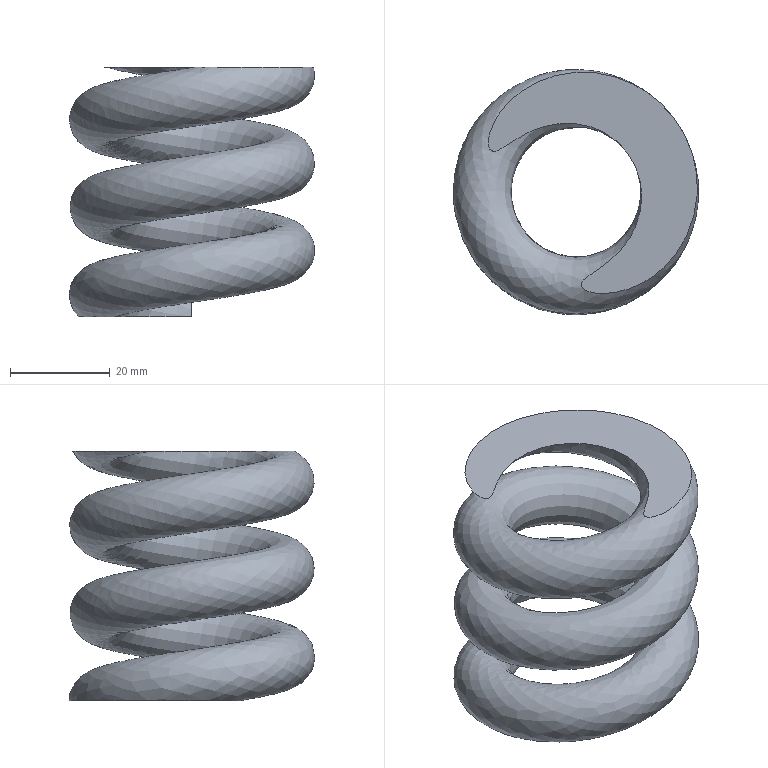Part | NX | features solid 2 | 1 solid | 4 faces | box 49.086 x 49.16 x 50 mm | volume 34729 mm3 | plane 3 | spline 1
STEP:
#1=CARTESIAN_POINT('',(849.833,314.642,270.));
#2=VERTEX_POINT('',#1);
#3=CARTESIAN_POINT('',(849.833,302.924,270.));
#4=VERTEX_POINT('',#3);
#5=CARTESIAN_POINT('',(849.833,308.783,270.));
#6=DIRECTION('',(1.,0.,0.));
#7=DIRECTION('',(0.,1.,0.));
#8=AXIS2_PLACEMENT_3D('',#5,#6,#7);
#9=CIRCLE('',#8,5.859);
#10=EDGE_CURVE('',#2,#4,#9,.T.);
#11=ORIENTED_EDGE('',*,*,#10,.F.);
#12=CARTESIAN_POINT('',(849.833,314.642,270.));
#13=CARTESIAN_POINT('',(846.44,314.642,270.));
#14=CARTESIAN_POINT('',(841.497,313.333,270.));
#15=CARTESIAN_POINT('',(835.698,309.831,270.));
#16=CARTESIAN_POINT('',(832.022,306.429,270.));
#17=CARTESIAN_POINT('',(829.182,302.192,270.));
#18=CARTESIAN_POINT('',(827.469,297.451,270.));
#19=CARTESIAN_POINT('',(826.996,293.248,270.));
#20=CARTESIAN_POINT('',(827.249,289.884,270.));
#21=CARTESIAN_POINT('',(827.774,287.404,270.));
#22=CARTESIAN_POINT('',(828.662,285.037,270.));
#23=CARTESIAN_POINT('',(829.739,283.199,270.));
#24=CARTESIAN_POINT('',(830.833,281.893,270.));
#25=CARTESIAN_POINT('',(831.626,281.182,270.));
#26=CARTESIAN_POINT('',(832.358,280.738,270.));
#27=CARTESIAN_POINT('',(832.958,280.513,270.));
#28=CARTESIAN_POINT('',(833.633,280.539,270.));
#29=CARTESIAN_POINT('',(834.101,281.032,270.));
#30=CARTESIAN_POINT('',(834.296,281.645,270.));
#31=CARTESIAN_POINT('',(834.427,282.48,270.));
#32=CARTESIAN_POINT('',(834.466,283.544,270.));
#33=CARTESIAN_POINT('',(834.481,284.816,270.));
#34=CARTESIAN_POINT('',(834.52,286.512,270.));
#35=CARTESIAN_POINT('',(834.693,288.633,270.));
#36=CARTESIAN_POINT('',(835.186,291.099,270.));
#37=CARTESIAN_POINT('',(836.003,293.489,270.));
#38=CARTESIAN_POINT('',(837.548,296.523,270.));
#39=CARTESIAN_POINT('',(840.241,299.847,270.));
#40=CARTESIAN_POINT('',(844.728,302.418,270.));
#41=CARTESIAN_POINT('',(848.126,302.924,270.));
#42=CARTESIAN_POINT('',(849.833,302.924,270.));
#43=B_SPLINE_CURVE_WITH_KNOTS('',3,(#12,#13,#14,#15,#16,#17,#18,#19,#20,#21,#22,#23,#24,#25,#26,#27,#28,#29,#30,#31,#32,#33,#34,#35,#36,#37,#38,#39,#40,#41,#42),.UNSPECIFIED.,.F.,.F.,(4,1,1,1,1,1,1,1,1,1,1,1,1,1,1,1,1,1,1,1,1,1,1,1,1,1,1,1,4),(0.,0.01003,0.01504,0.02005,0.02507,0.03008,0.03509,0.0376,0.04011,0.04261,0.04512,0.04637,0.04763,0.04825,0.04888,0.04951,0.05013,0.05076,0.05139,0.05264,0.05389,0.05515,0.05765,0.06016,0.06267,0.06517,0.07019,0.0752,0.08021),.UNSPECIFIED.);
#44=EDGE_CURVE('',#2,#4,#43,.T.);
#45=ORIENTED_EDGE('',*,*,#44,.T.);
#46=EDGE_LOOP('',(#11,#45));
#47=FACE_BOUND('',#46,.T.);
#48=CARTESIAN_POINT('',(832.448,298.878,320.));
#49=VERTEX_POINT('',#48);
#50=CARTESIAN_POINT('',(832.254,300.141,320.));
#51=CARTESIAN_POINT('',(832.305,299.07,320.));
#52=CARTESIAN_POINT('',(832.744,298.28,320.));
#53=CARTESIAN_POINT('',(833.397,298.073,320.));
#54=CARTESIAN_POINT('',(834.032,298.232,320.));
#55=CARTESIAN_POINT('',(834.812,298.582,320.));
#56=CARTESIAN_POINT('',(835.715,299.141,320.));
#57=CARTESIAN_POINT('',(837.137,300.078,320.));
#58=CARTESIAN_POINT('',(838.937,301.205,320.));
#59=CARTESIAN_POINT('',(841.207,302.322,320.));
#60=CARTESIAN_POINT('',(843.631,303.17,320.));
#61=CARTESIAN_POINT('',(846.975,303.843,320.));
#62=CARTESIAN_POINT('',(851.29,303.731,320.));
#63=CARTESIAN_POINT('',(856.125,301.869,320.));
#64=CARTESIAN_POINT('',(860.038,298.458,320.));
#65=CARTESIAN_POINT('',(862.508,293.89,320.));
#66=CARTESIAN_POINT('',(863.31,288.76,320.));
#67=CARTESIAN_POINT('',(862.43,284.528,320.));
#68=CARTESIAN_POINT('',(861.007,281.414,320.));
#69=CARTESIAN_POINT('',(859.591,279.276,320.));
#70=CARTESIAN_POINT('',(857.882,277.383,320.));
#71=CARTESIAN_POINT('',(855.93,275.7,320.));
#72=CARTESIAN_POINT('',(854.187,274.474,320.));
#73=CARTESIAN_POINT('',(852.769,273.521,320.));
#74=CARTESIAN_POINT('',(851.898,272.903,320.));
#75=CARTESIAN_POINT('',(851.273,272.322,320.));
#76=CARTESIAN_POINT('',(850.88,271.795,320.));
#77=CARTESIAN_POINT('',(850.86,271.109,320.));
#78=CARTESIAN_POINT('',(851.466,270.444,320.));
#79=CARTESIAN_POINT('',(852.449,270.02,320.));
#80=CARTESIAN_POINT('',(853.701,269.748,320.));
#81=CARTESIAN_POINT('',(854.962,269.656,320.));
#82=CARTESIAN_POINT('',(856.651,269.707,320.));
#83=CARTESIAN_POINT('',(858.744,270.054,320.));
#84=CARTESIAN_POINT('',(861.135,270.817,320.));
#85=CARTESIAN_POINT('',(864.203,272.267,320.));
#86=CARTESIAN_POINT('',(867.616,274.777,320.));
#87=CARTESIAN_POINT('',(870.808,278.704,320.));
#88=CARTESIAN_POINT('',(873.006,283.281,320.));
#89=CARTESIAN_POINT('',(874.143,288.233,320.));
#90=CARTESIAN_POINT('',(874.232,294.958,320.));
#91=CARTESIAN_POINT('',(871.48,303.132,320.));
#92=CARTESIAN_POINT('',(865.584,309.311,320.));
#93=CARTESIAN_POINT('',(859.611,312.508,320.));
#94=CARTESIAN_POINT('',(854.779,313.872,320.));
#95=CARTESIAN_POINT('',(849.707,314.128,320.));
#96=CARTESIAN_POINT('',(844.723,313.19,320.));
#97=CARTESIAN_POINT('',(840.893,311.506,320.));
#98=CARTESIAN_POINT('',(838.089,309.59,320.));
#99=CARTESIAN_POINT('',(836.219,307.921,320.));
#100=CARTESIAN_POINT('',(834.576,305.984,320.));
#101=CARTESIAN_POINT('',(833.481,304.18,320.));
#102=CARTESIAN_POINT('',(832.815,302.623,320.));
#103=CARTESIAN_POINT('',(832.444,301.403,320.));
#104=CARTESIAN_POINT('',(832.254,300.141,320.));
#105=CARTESIAN_POINT('',(832.305,299.07,320.));
#106=CARTESIAN_POINT('',(832.744,298.28,320.));
#107=B_SPLINE_CURVE_WITH_KNOTS('',3,(#50,#51,#52,#53,#54,#55,#56,#57,#58,#59,#60,#61,#62,#63,#64,#65,#66,#67,#68,#69,#70,#71,#72,#73,#74,#75,#76,#77,#78,#79,#80,#81,#82,#83,#84,#85,#86,#87,#88,#89,#90,#91,#92,#93,#94,#95,#96,#97,#98,#99,#100,#101,#102,#103,#104,#105,#106),.UNSPECIFIED.,.T.,.F.,(1,1,1,1,1,1,1,1,1,1,1,1,1,1,1,1,1,1,1,1,1,1,1,1,1,1,1,1,1,1,1,1,1,1,1,1,1,1,1,1,1,1,1,1,1,1,1,1,1,1,1,1,1,1,1,1,1,1,1,1,1),(-0.003862,-0.002575,-0.001287,0.,0.0006437,0.001287,0.001931,0.002575,0.003862,0.00515,0.007725,0.0103,0.01287,0.01545,0.0206,0.02575,0.0309,0.03605,0.0412,0.04635,0.04892,0.0515,0.05407,0.05665,0.05922,0.06051,0.0618,0.06244,0.06308,0.06373,0.06437,0.06566,0.06695,0.06823,0.06952,0.0721,0.07467,0.07725,0.0824,0.08755,0.0927,0.09785,0.103,0.1133,0.1236,0.1287,0.1339,0.139,0.1442,0.1493,0.1519,0.1545,0.1571,0.1596,0.1609,0.1622,0.1635,0.1648,0.1654,0.1661,0.1667),.UNSPECIFIED.);
#108=EDGE_CURVE('',#49,#49,#107,.T.);
#109=ORIENTED_EDGE('',*,*,#108,.F.);
#110=EDGE_LOOP('',(#109));
#111=FACE_BOUND('',#110,.T.);
#112=CARTESIAN_POINT('',(849.833,314.642,267.928));
#113=CARTESIAN_POINT('',(842.8,314.642,268.978));
#114=CARTESIAN_POINT('',(831.674,309.421,270.651));
#115=CARTESIAN_POINT('',(825.098,296.53,272.763));
#116=CARTESIAN_POINT('',(824.615,287.249,274.119));
#117=CARTESIAN_POINT('',(826.656,280.376,275.182));
#118=CARTESIAN_POINT('',(830.072,274.109,276.24));
#119=CARTESIAN_POINT('',(836.949,267.835,277.601));
#120=CARTESIAN_POINT('',(847.495,264.445,279.212));
#121=CARTESIAN_POINT('',(858.422,265.955,280.824));
#122=CARTESIAN_POINT('',(867.75,271.807,282.428));
#123=CARTESIAN_POINT('',(873.583,281.1,284.026));
#124=CARTESIAN_POINT('',(875.079,291.906,285.619));
#125=CARTESIAN_POINT('',(871.753,302.261,287.201));
#126=CARTESIAN_POINT('',(864.508,310.205,288.773));
#127=CARTESIAN_POINT('',(851.467,315.65,290.825));
#128=CARTESIAN_POINT('',(833.203,310.78,293.401));
#129=CARTESIAN_POINT('',(823.842,290.7,296.408));
#130=CARTESIAN_POINT('',(832.981,271.086,299.345));
#131=CARTESIAN_POINT('',(850.033,266.535,301.75));
#132=CARTESIAN_POINT('',(861.836,271.46,303.607));
#133=CARTESIAN_POINT('',(868.201,278.435,304.988));
#134=CARTESIAN_POINT('',(871.051,287.302,306.342));
#135=CARTESIAN_POINT('',(869.8,296.353,307.677));
#136=CARTESIAN_POINT('',(865.031,303.955,308.984));
#137=CARTESIAN_POINT('',(857.571,308.637,310.267));
#138=CARTESIAN_POINT('',(849.024,309.821,311.527));
#139=CARTESIAN_POINT('',(840.959,307.23,312.759));
#140=CARTESIAN_POINT('',(835.856,302.576,313.769));
#141=CARTESIAN_POINT('',(833.291,297.873,314.563));
#142=CARTESIAN_POINT('',(831.783,292.799,315.348));
#143=CARTESIAN_POINT('',(832.124,286.217,316.31));
#144=CARTESIAN_POINT('',(836.848,276.966,317.826));
#145=CARTESIAN_POINT('',(848.976,271.282,319.645));
#146=CARTESIAN_POINT('',(860.666,276.758,321.398));
#147=CARTESIAN_POINT('',(864.966,285.174,322.777));
#148=CARTESIAN_POINT('',(865.26,290.821,323.602));
#149=CARTESIAN_POINT('',(863.986,295.111,324.265));
#150=CARTESIAN_POINT('',(861.867,298.998,324.922));
#151=CARTESIAN_POINT('',(857.875,302.64,325.712));
#152=CARTESIAN_POINT('',(851.736,304.613,326.65));
#153=CARTESIAN_POINT('',(845.458,303.746,327.576));
#154=CARTESIAN_POINT('',(840.305,300.513,328.462));
#155=CARTESIAN_POINT('',(838.163,297.214,329.037));
#156=CARTESIAN_POINT('',(837.477,295.499,329.312));
#157=CARTESIAN_POINT('',(849.833,314.642,272.072));
#158=CARTESIAN_POINT('',(843.407,314.642,273.03));
#159=CARTESIAN_POINT('',(832.438,309.495,274.68));
#160=CARTESIAN_POINT('',(826.013,296.9,276.743));
#161=CARTESIAN_POINT('',(825.547,287.951,278.051));
#162=CARTESIAN_POINT('',(827.506,281.357,279.07));
#163=CARTESIAN_POINT('',(830.764,275.38,280.08));
#164=CARTESIAN_POINT('',(837.245,269.466,281.363));
#165=CARTESIAN_POINT('',(847.107,266.296,282.869));
#166=CARTESIAN_POINT('',(857.228,267.695,284.362));
#167=CARTESIAN_POINT('',(865.779,273.059,285.832));
#168=CARTESIAN_POINT('',(871.074,281.496,287.283));
#169=CARTESIAN_POINT('',(872.419,291.211,288.716));
#170=CARTESIAN_POINT('',(869.458,300.427,290.123));
#171=CARTESIAN_POINT('',(863.062,307.442,291.512));
#172=CARTESIAN_POINT('',(851.607,312.224,293.314));
#173=CARTESIAN_POINT('',(835.916,308.04,295.527));
#174=CARTESIAN_POINT('',(827.949,290.951,298.086));
#175=CARTESIAN_POINT('',(835.612,274.505,300.549));
#176=CARTESIAN_POINT('',(849.634,270.762,302.526));
#177=CARTESIAN_POINT('',(859.381,274.83,304.06));
#178=CARTESIAN_POINT('',(864.564,280.51,305.184));
#179=CARTESIAN_POINT('',(866.867,287.676,306.279));
#180=CARTESIAN_POINT('',(865.859,294.971,307.355));
#181=CARTESIAN_POINT('',(862.029,301.076,308.404));
#182=CARTESIAN_POINT('',(856.052,304.828,309.432));
#183=CARTESIAN_POINT('',(849.212,305.775,310.441));
#184=CARTESIAN_POINT('',(842.771,303.706,311.425));
#185=CARTESIAN_POINT('',(838.734,300.024,312.224));
#186=CARTESIAN_POINT('',(836.65,296.203,312.869));
#187=CARTESIAN_POINT('',(835.427,292.088,313.505));
#188=CARTESIAN_POINT('',(835.698,286.86,314.27));
#189=CARTESIAN_POINT('',(839.567,279.284,315.511));
#190=CARTESIAN_POINT('',(849.375,274.686,316.982));
#191=CARTESIAN_POINT('',(858.951,279.172,318.418));
#192=CARTESIAN_POINT('',(862.594,286.303,319.586));
#193=CARTESIAN_POINT('',(862.841,291.033,320.278));
#194=CARTESIAN_POINT('',(861.743,294.73,320.849));
#195=CARTESIAN_POINT('',(859.897,298.117,321.421));
#196=CARTESIAN_POINT('',(856.452,301.259,322.103));
#197=CARTESIAN_POINT('',(851.037,303.,322.93));
#198=CARTESIAN_POINT('',(845.407,302.222,323.761));
#199=CARTESIAN_POINT('',(840.705,299.272,324.569));
#200=CARTESIAN_POINT('',(838.718,296.21,325.103));
#201=CARTESIAN_POINT('',(838.079,294.604,325.36));
#202=CARTESIAN_POINT('',(849.833,313.607,274.824));
#203=CARTESIAN_POINT('',(844.036,313.607,275.688));
#204=CARTESIAN_POINT('',(833.689,308.751,277.245));
#205=CARTESIAN_POINT('',(827.618,296.848,279.194));
#206=CARTESIAN_POINT('',(827.183,288.501,280.415));
#207=CARTESIAN_POINT('',(829.009,282.352,281.365));
#208=CARTESIAN_POINT('',(832.036,276.8,282.302));
#209=CARTESIAN_POINT('',(837.985,271.372,283.48));
#210=CARTESIAN_POINT('',(846.999,268.474,284.857));
#211=CARTESIAN_POINT('',(856.188,269.745,286.212));
#212=CARTESIAN_POINT('',(863.897,274.58,287.538));
#213=CARTESIAN_POINT('',(868.639,282.135,288.837));
#214=CARTESIAN_POINT('',(869.835,290.777,290.111));
#215=CARTESIAN_POINT('',(867.22,298.918,291.355));
#216=CARTESIAN_POINT('',(861.596,305.085,292.576));
#217=CARTESIAN_POINT('',(851.535,309.286,294.158));
#218=CARTESIAN_POINT('',(838.002,305.677,296.067));
#219=CARTESIAN_POINT('',(831.149,290.978,298.268));
#220=CARTESIAN_POINT('',(837.689,276.941,300.37));
#221=CARTESIAN_POINT('',(849.504,273.788,302.037));
#222=CARTESIAN_POINT('',(857.807,277.253,303.343));
#223=CARTESIAN_POINT('',(862.18,282.045,304.292));
#224=CARTESIAN_POINT('',(864.118,288.075,305.212));
#225=CARTESIAN_POINT('',(863.268,294.225,306.119));
#226=CARTESIAN_POINT('',(860.036,299.379,307.006));
#227=CARTESIAN_POINT('',(854.977,302.553,307.876));
#228=CARTESIAN_POINT('',(849.166,303.358,308.733));
#229=CARTESIAN_POINT('',(843.675,301.594,309.571));
#230=CARTESIAN_POINT('',(840.244,298.465,310.25));
#231=CARTESIAN_POINT('',(838.426,295.132,310.813));
#232=CARTESIAN_POINT('',(837.357,291.537,311.369));
#233=CARTESIAN_POINT('',(837.592,287.022,312.029));
#234=CARTESIAN_POINT('',(841.03,280.288,313.132));
#235=CARTESIAN_POINT('',(849.757,276.198,314.441));
#236=CARTESIAN_POINT('',(858.446,280.268,315.744));
#237=CARTESIAN_POINT('',(861.849,286.928,316.835));
#238=CARTESIAN_POINT('',(862.08,291.362,317.484));
#239=CARTESIAN_POINT('',(861.032,294.89,318.029));
#240=CARTESIAN_POINT('',(859.254,298.152,318.58));
#241=CARTESIAN_POINT('',(855.92,301.193,319.24));
#242=CARTESIAN_POINT('',(850.597,302.905,320.053));
#243=CARTESIAN_POINT('',(844.983,302.129,320.881));
#244=CARTESIAN_POINT('',(840.227,299.145,321.699));
#245=CARTESIAN_POINT('',(838.191,296.006,322.245));
#246=CARTESIAN_POINT('',(837.535,294.349,322.511));
#247=CARTESIAN_POINT('',(849.833,310.855,275.859));
#248=CARTESIAN_POINT('',(844.788,310.855,276.612));
#249=CARTESIAN_POINT('',(835.856,306.663,277.955));
#250=CARTESIAN_POINT('',(830.494,296.152,279.677));
#251=CARTESIAN_POINT('',(830.117,288.898,280.737));
#252=CARTESIAN_POINT('',(831.717,283.51,281.57));
#253=CARTESIAN_POINT('',(834.368,278.647,282.391));
#254=CARTESIAN_POINT('',(839.5,273.964,283.408));
#255=CARTESIAN_POINT('',(847.297,271.458,284.598));
#256=CARTESIAN_POINT('',(855.237,272.555,285.769));
#257=CARTESIAN_POINT('',(861.885,276.726,286.912));
#258=CARTESIAN_POINT('',(865.97,283.234,288.032));
#259=CARTESIAN_POINT('',(867.,290.678,289.13));
#260=CARTESIAN_POINT('',(864.749,297.686,290.2));
#261=CARTESIAN_POINT('',(859.894,303.01,291.254));
#262=CARTESIAN_POINT('',(851.132,306.669,292.632));
#263=CARTESIAN_POINT('',(839.436,303.55,294.282));
#264=CARTESIAN_POINT('',(833.431,290.67,296.211));
#265=CARTESIAN_POINT('',(839.225,278.235,298.072));
#266=CARTESIAN_POINT('',(849.763,275.422,299.559));
#267=CARTESIAN_POINT('',(857.343,278.585,300.751));
#268=CARTESIAN_POINT('',(861.356,282.984,301.622));
#269=CARTESIAN_POINT('',(863.152,288.57,302.475));
#270=CARTESIAN_POINT('',(862.355,294.336,303.326));
#271=CARTESIAN_POINT('',(859.286,299.229,304.167));
#272=CARTESIAN_POINT('',(854.422,302.281,305.003));
#273=CARTESIAN_POINT('',(848.757,303.066,305.839));
#274=CARTESIAN_POINT('',(843.331,301.323,306.667));
#275=CARTESIAN_POINT('',(839.894,298.188,307.348));
#276=CARTESIAN_POINT('',(838.056,294.819,307.917));
#277=CARTESIAN_POINT('',(836.966,291.15,308.484));
#278=CARTESIAN_POINT('',(837.208,286.477,309.167));
#279=CARTESIAN_POINT('',(840.799,279.446,310.319));
#280=CARTESIAN_POINT('',(850.164,275.056,311.724));
#281=CARTESIAN_POINT('',(859.701,279.524,313.154));
#282=CARTESIAN_POINT('',(863.459,286.879,314.359));
#283=CARTESIAN_POINT('',(863.722,291.917,315.096));
#284=CARTESIAN_POINT('',(862.541,295.891,315.71));
#285=CARTESIAN_POINT('',(860.53,299.58,316.333));
#286=CARTESIAN_POINT('',(856.662,303.11,317.099));
#287=CARTESIAN_POINT('',(850.486,305.095,318.042));
#288=CARTESIAN_POINT('',(843.937,304.189,319.008));
#289=CARTESIAN_POINT('',(838.353,300.687,319.968));
#290=CARTESIAN_POINT('',(835.952,296.985,320.613));
#291=CARTESIAN_POINT('',(835.178,295.026,320.927));
#292=CARTESIAN_POINT('',(849.833,306.711,275.859));
#293=CARTESIAN_POINT('',(845.693,306.711,276.477));
#294=CARTESIAN_POINT('',(838.831,303.491,277.509));
#295=CARTESIAN_POINT('',(834.481,294.964,278.906));
#296=CARTESIAN_POINT('',(834.183,289.232,279.744));
#297=CARTESIAN_POINT('',(835.474,284.886,280.415));
#298=CARTESIAN_POINT('',(837.62,280.948,281.08));
#299=CARTESIAN_POINT('',(841.67,277.253,281.882));
#300=CARTESIAN_POINT('',(847.893,275.253,282.833));
#301=CARTESIAN_POINT('',(854.253,276.132,283.771));
#302=CARTESIAN_POINT('',(859.597,279.484,284.689));
#303=CARTESIAN_POINT('',(862.895,284.74,285.593));
#304=CARTESIAN_POINT('',(863.733,290.791,286.486));
#305=CARTESIAN_POINT('',(861.893,296.521,287.361));
#306=CARTESIAN_POINT('',(857.875,300.926,288.233));
#307=CARTESIAN_POINT('',(850.471,304.018,289.397));
#308=CARTESIAN_POINT('',(840.573,301.378,290.794));
#309=CARTESIAN_POINT('',(835.32,290.111,292.481));
#310=CARTESIAN_POINT('',(840.545,278.896,294.16));
#311=CARTESIAN_POINT('',(850.304,276.291,295.537));
#312=CARTESIAN_POINT('',(857.567,279.322,296.679));
#313=CARTESIAN_POINT('',(861.484,283.615,297.529));
#314=CARTESIAN_POINT('',(863.271,289.174,298.378));
#315=CARTESIAN_POINT('',(862.463,295.024,299.241));
#316=CARTESIAN_POINT('',(859.287,300.087,300.111));
#317=CARTESIAN_POINT('',(854.158,303.306,300.993));
#318=CARTESIAN_POINT('',(848.071,304.149,301.891));
#319=CARTESIAN_POINT('',(842.132,302.241,302.798));
#320=CARTESIAN_POINT('',(838.285,298.732,303.56));
#321=CARTESIAN_POINT('',(836.235,294.975,304.194));
#322=CARTESIAN_POINT('',(835.005,290.835,304.834));
#323=CARTESIAN_POINT('',(835.286,285.414,305.627));
#324=CARTESIAN_POINT('',(839.427,277.305,306.955));
#325=CARTESIAN_POINT('',(850.627,272.056,308.635));
#326=CARTESIAN_POINT('',(862.236,277.494,310.376));
#327=CARTESIAN_POINT('',(866.776,286.379,311.832));
#328=CARTESIAN_POINT('',(867.104,292.671,312.752));
#329=CARTESIAN_POINT('',(865.657,297.542,313.505));
#330=CARTESIAN_POINT('',(863.194,302.061,314.268));
#331=CARTESIAN_POINT('',(858.313,306.514,315.234));
#332=CARTESIAN_POINT('',(850.582,308.999,316.415));
#333=CARTESIAN_POINT('',(842.38,307.865,317.624));
#334=CARTESIAN_POINT('',(835.381,303.475,318.828));
#335=CARTESIAN_POINT('',(832.372,298.836,319.636));
#336=CARTESIAN_POINT('',(831.402,296.384,320.029));
#337=CARTESIAN_POINT('',(849.833,303.959,274.824));
#338=CARTESIAN_POINT('',(846.142,303.959,275.374));
#339=CARTESIAN_POINT('',(840.616,301.366,276.205));
#340=CARTESIAN_POINT('',(836.901,294.083,277.398));
#341=CARTESIAN_POINT('',(836.651,289.278,278.101));
#342=CARTESIAN_POINT('',(837.757,285.554,278.676));
#343=CARTESIAN_POINT('',(839.607,282.16,279.249));
#344=CARTESIAN_POINT('',(843.037,279.03,279.929));
#345=CARTESIAN_POINT('',(848.385,277.311,280.745));
#346=CARTESIAN_POINT('',(853.898,278.073,281.558));
#347=CARTESIAN_POINT('',(858.57,281.003,282.362));
#348=CARTESIAN_POINT('',(861.481,285.642,283.159));
#349=CARTESIAN_POINT('',(862.228,291.04,283.955));
#350=CARTESIAN_POINT('',(860.569,296.205,284.744));
#351=CARTESIAN_POINT('',(856.896,300.233,285.542));
#352=CARTESIAN_POINT('',(849.997,303.113,286.627));
#353=CARTESIAN_POINT('',(840.65,300.621,287.945));
#354=CARTESIAN_POINT('',(835.548,289.677,289.584));
#355=CARTESIAN_POINT('',(840.765,278.48,291.261));
#356=CARTESIAN_POINT('',(850.763,275.812,292.671));
#357=CARTESIAN_POINT('',(858.33,278.969,293.861));
#358=CARTESIAN_POINT('',(862.479,283.516,294.761));
#359=CARTESIAN_POINT('',(864.397,289.482,295.672));
#360=CARTESIAN_POINT('',(863.52,295.826,296.608));
#361=CARTESIAN_POINT('',(860.038,301.376,297.562));
#362=CARTESIAN_POINT('',(854.362,304.938,298.538));
#363=CARTESIAN_POINT('',(847.568,305.879,299.541));
#364=CARTESIAN_POINT('',(840.882,303.732,300.561));
#365=CARTESIAN_POINT('',(836.496,299.732,301.43));
#366=CARTESIAN_POINT('',(834.186,295.496,302.145));
#367=CARTESIAN_POINT('',(832.791,290.804,302.87));
#368=CARTESIAN_POINT('',(833.116,284.548,303.785));
#369=CARTESIAN_POINT('',(837.836,275.304,305.299));
#370=CARTESIAN_POINT('',(850.834,269.211,307.249));
#371=CARTESIAN_POINT('',(864.349,275.543,309.276));
#372=CARTESIAN_POINT('',(869.572,285.765,310.951));
#373=CARTESIAN_POINT('',(869.955,293.119,312.026));
#374=CARTESIAN_POINT('',(868.288,298.734,312.894));
#375=CARTESIAN_POINT('',(865.456,303.929,313.771));
#376=CARTESIAN_POINT('',(859.766,309.12,314.898));
#377=CARTESIAN_POINT('',(850.82,311.996,316.264));
#378=CARTESIAN_POINT('',(841.359,310.688,317.659));
#379=CARTESIAN_POINT('',(833.306,305.637,319.044));
#380=CARTESIAN_POINT('',(829.855,300.317,319.971));
#381=CARTESIAN_POINT('',(828.743,297.509,320.421));
#382=CARTESIAN_POINT('',(849.833,302.924,272.072));
#383=CARTESIAN_POINT('',(845.965,302.924,272.649));
#384=CARTESIAN_POINT('',(840.852,300.524,273.418));
#385=CARTESIAN_POINT('',(837.29,293.54,274.562));
#386=CARTESIAN_POINT('',(837.048,288.896,275.241));
#387=CARTESIAN_POINT('',(838.132,285.246,275.805));
#388=CARTESIAN_POINT('',(839.961,281.891,276.371));
#389=CARTESIAN_POINT('',(843.382,278.769,277.049));
#390=CARTESIAN_POINT('',(848.791,277.03,277.875));
#391=CARTESIAN_POINT('',(854.446,277.812,278.709));
#392=CARTESIAN_POINT('',(859.307,280.861,279.545));
#393=CARTESIAN_POINT('',(862.378,285.755,280.386));
#394=CARTESIAN_POINT('',(863.178,291.53,281.238));
#395=CARTESIAN_POINT('',(861.379,297.132,282.093));
#396=CARTESIAN_POINT('',(857.352,301.547,282.967));
#397=CARTESIAN_POINT('',(849.739,304.726,284.165));
#398=CARTESIAN_POINT('',(839.132,301.898,285.661));
#399=CARTESIAN_POINT('',(833.292,289.371,287.537));
#400=CARTESIAN_POINT('',(839.347,276.375,289.483));
#401=CARTESIAN_POINT('',(851.164,273.221,291.15));
#402=CARTESIAN_POINT('',(860.016,276.915,292.542));
#403=CARTESIAN_POINT('',(864.926,282.297,293.608));
#404=CARTESIAN_POINT('',(867.205,289.385,294.69));
#405=CARTESIAN_POINT('',(866.164,296.916,295.801));
#406=CARTESIAN_POINT('',(862.032,303.503,296.933));
#407=CARTESIAN_POINT('',(855.305,307.725,298.09));
#408=CARTESIAN_POINT('',(847.271,308.837,299.275));
#409=CARTESIAN_POINT('',(839.379,306.302,300.48));
#410=CARTESIAN_POINT('',(834.182,301.563,301.509));
#411=CARTESIAN_POINT('',(831.5,296.645,302.34));
#412=CARTESIAN_POINT('',(829.88,291.197,303.182));
#413=CARTESIAN_POINT('',(830.262,283.855,304.255));
#414=CARTESIAN_POINT('',(835.687,273.23,305.996));
#415=CARTESIAN_POINT('',(850.685,266.2,308.245));
#416=CARTESIAN_POINT('',(866.122,273.432,310.561));
#417=CARTESIAN_POINT('',(871.976,284.89,312.438));
#418=CARTESIAN_POINT('',(872.408,293.166,313.648));
#419=CARTESIAN_POINT('',(870.556,299.4,314.611));
#420=CARTESIAN_POINT('',(867.43,305.135,315.58));
#421=CARTESIAN_POINT('',(861.124,310.888,316.829));
#422=CARTESIAN_POINT('',(851.308,314.044,318.328));
#423=CARTESIAN_POINT('',(841.004,312.619,319.847));
#424=CARTESIAN_POINT('',(832.297,307.158,321.344));
#425=CARTESIAN_POINT('',(828.592,301.446,322.339));
#426=CARTESIAN_POINT('',(827.399,298.443,322.821));
#427=CARTESIAN_POINT('',(849.833,302.924,267.928));
#428=CARTESIAN_POINT('',(845.358,302.924,268.596));
#429=CARTESIAN_POINT('',(840.088,300.45,269.389));
#430=CARTESIAN_POINT('',(836.374,293.17,270.581));
#431=CARTESIAN_POINT('',(836.115,288.194,271.309));
#432=CARTESIAN_POINT('',(837.282,284.265,271.916));
#433=CARTESIAN_POINT('',(839.27,280.62,272.531));
#434=CARTESIAN_POINT('',(843.086,277.138,273.287));
#435=CARTESIAN_POINT('',(849.179,275.179,274.218));
#436=CARTESIAN_POINT('',(855.64,276.072,275.17));
#437=CARTESIAN_POINT('',(861.278,279.609,276.14));
#438=CARTESIAN_POINT('',(864.887,285.359,277.129));
#439=CARTESIAN_POINT('',(865.838,292.226,278.141));
#440=CARTESIAN_POINT('',(863.673,298.965,279.171));
#441=CARTESIAN_POINT('',(858.798,304.311,280.229));
#442=CARTESIAN_POINT('',(849.599,308.152,281.676));
#443=CARTESIAN_POINT('',(836.419,304.637,283.535));
#444=CARTESIAN_POINT('',(829.185,289.12,285.859));
#445=CARTESIAN_POINT('',(836.716,272.956,288.279));
#446=CARTESIAN_POINT('',(851.563,268.993,290.373));
#447=CARTESIAN_POINT('',(862.471,273.545,292.089));
#448=CARTESIAN_POINT('',(868.563,280.222,293.411));
#449=CARTESIAN_POINT('',(871.389,289.011,294.753));
#450=CARTESIAN_POINT('',(870.105,298.298,296.123));
#451=CARTESIAN_POINT('',(865.034,306.382,297.513));
#452=CARTESIAN_POINT('',(856.824,311.534,298.925));
#453=CARTESIAN_POINT('',(847.083,312.883,300.362));
#454=CARTESIAN_POINT('',(837.567,309.827,301.815));
#455=CARTESIAN_POINT('',(831.304,304.115,303.054));
#456=CARTESIAN_POINT('',(828.141,298.316,304.034));
#457=CARTESIAN_POINT('',(826.236,291.908,305.024));
#458=CARTESIAN_POINT('',(826.688,283.212,306.296));
#459=CARTESIAN_POINT('',(832.969,270.912,308.311));
#460=CARTESIAN_POINT('',(850.285,262.795,310.908));
#461=CARTESIAN_POINT('',(867.837,271.018,313.54));
#462=CARTESIAN_POINT('',(874.347,283.76,315.628));
#463=CARTESIAN_POINT('',(874.827,292.954,316.973));
#464=CARTESIAN_POINT('',(872.799,299.781,318.027));
#465=CARTESIAN_POINT('',(869.4,306.016,319.081));
#466=CARTESIAN_POINT('',(862.547,312.269,320.438));
#467=CARTESIAN_POINT('',(852.007,315.657,322.047));
#468=CARTESIAN_POINT('',(841.056,314.143,323.662));
#469=CARTESIAN_POINT('',(831.897,308.399,325.237));
#470=CARTESIAN_POINT('',(828.037,302.45,326.273));
#471=CARTESIAN_POINT('',(826.797,299.339,326.773));
#472=CARTESIAN_POINT('',(849.833,303.959,265.176));
#473=CARTESIAN_POINT('',(844.729,303.959,265.938));
#474=CARTESIAN_POINT('',(838.837,301.194,266.824));
#475=CARTESIAN_POINT('',(834.77,293.222,268.13));
#476=CARTESIAN_POINT('',(834.479,287.644,268.945));
#477=CARTESIAN_POINT('',(835.779,283.27,269.621));
#478=CARTESIAN_POINT('',(837.997,279.2,270.309));
#479=CARTESIAN_POINT('',(842.346,275.232,271.17));
#480=CARTESIAN_POINT('',(849.287,273.001,272.23));
#481=CARTESIAN_POINT('',(856.679,274.023,273.32));
#482=CARTESIAN_POINT('',(863.16,278.088,274.434));
#483=CARTESIAN_POINT('',(867.322,284.72,275.575));
#484=CARTESIAN_POINT('',(868.422,292.659,276.746));
#485=CARTESIAN_POINT('',(865.911,300.474,277.939));
#486=CARTESIAN_POINT('',(860.263,306.668,279.165));
#487=CARTESIAN_POINT('',(849.671,311.09,280.831));
#488=CARTESIAN_POINT('',(834.333,307.,282.995));
#489=CARTESIAN_POINT('',(825.985,289.093,285.676));
#490=CARTESIAN_POINT('',(834.639,270.52,288.457));
#491=CARTESIAN_POINT('',(851.694,265.968,290.863));
#492=CARTESIAN_POINT('',(864.045,271.122,292.806));
#493=CARTESIAN_POINT('',(870.947,278.687,294.304));
#494=CARTESIAN_POINT('',(874.138,288.612,295.82));
#495=CARTESIAN_POINT('',(872.696,299.044,297.358));
#496=CARTESIAN_POINT('',(867.028,308.08,298.912));
#497=CARTESIAN_POINT('',(857.899,313.809,300.482));
#498=CARTESIAN_POINT('',(847.129,315.3,302.07));
#499=CARTESIAN_POINT('',(836.664,311.938,303.668));
#500=CARTESIAN_POINT('',(829.795,305.674,305.028));
#501=CARTESIAN_POINT('',(826.365,299.386,306.09));
#502=CARTESIAN_POINT('',(824.306,292.459,307.161));
#503=CARTESIAN_POINT('',(824.794,283.05,308.536));
#504=CARTESIAN_POINT('',(831.506,269.908,310.689));
#505=CARTESIAN_POINT('',(849.904,261.284,313.449));
#506=CARTESIAN_POINT('',(868.342,269.922,316.214));
#507=CARTESIAN_POINT('',(875.093,283.135,318.379));
#508=CARTESIAN_POINT('',(875.588,292.625,319.767));
#509=CARTESIAN_POINT('',(873.51,299.621,320.848));
#510=CARTESIAN_POINT('',(870.043,305.981,321.922));
#511=CARTESIAN_POINT('',(863.079,312.335,323.301));
#512=CARTESIAN_POINT('',(852.447,315.753,324.925));
#513=CARTESIAN_POINT('',(841.479,314.236,326.542));
#514=CARTESIAN_POINT('',(832.375,308.526,328.108));
#515=CARTESIAN_POINT('',(828.563,302.654,329.131));
#516=CARTESIAN_POINT('',(827.341,299.594,329.622));
#517=CARTESIAN_POINT('',(849.833,306.711,264.141));
#518=CARTESIAN_POINT('',(843.976,306.711,265.014));
#519=CARTESIAN_POINT('',(836.67,303.282,266.113));
#520=CARTESIAN_POINT('',(831.893,293.918,267.647));
#521=CARTESIAN_POINT('',(831.546,287.247,268.622));
#522=CARTESIAN_POINT('',(833.071,282.112,269.416));
#523=CARTESIAN_POINT('',(835.665,277.353,270.22));
#524=CARTESIAN_POINT('',(840.831,272.64,271.243));
#525=CARTESIAN_POINT('',(848.989,270.017,272.488));
#526=CARTESIAN_POINT('',(857.631,271.212,273.763));
#527=CARTESIAN_POINT('',(865.172,275.942,275.06));
#528=CARTESIAN_POINT('',(869.991,283.621,276.38));
#529=CARTESIAN_POINT('',(871.257,292.758,277.728));
#530=CARTESIAN_POINT('',(868.382,301.706,279.094));
#531=CARTESIAN_POINT('',(861.965,308.743,280.487));
#532=CARTESIAN_POINT('',(850.075,313.708,282.358));
#533=CARTESIAN_POINT('',(832.9,309.128,284.78));
#534=CARTESIAN_POINT('',(823.703,289.401,287.734));
#535=CARTESIAN_POINT('',(833.103,269.226,290.755));
#536=CARTESIAN_POINT('',(851.434,264.333,293.341));
#537=CARTESIAN_POINT('',(864.509,269.79,295.397));
#538=CARTESIAN_POINT('',(871.771,277.748,296.973));
#539=CARTESIAN_POINT('',(875.104,288.117,298.557));
#540=CARTESIAN_POINT('',(873.609,298.933,300.152));
#541=CARTESIAN_POINT('',(867.778,308.229,301.75));
#542=CARTESIAN_POINT('',(858.454,314.081,303.354));
#543=CARTESIAN_POINT('',(847.538,315.592,304.964));
#544=CARTESIAN_POINT('',(837.007,312.21,306.572));
#545=CARTESIAN_POINT('',(830.144,305.951,307.93));
#546=CARTESIAN_POINT('',(826.735,299.7,308.986));
#547=CARTESIAN_POINT('',(824.697,292.846,310.046));
#548=CARTESIAN_POINT('',(825.178,283.595,311.398));
#549=CARTESIAN_POINT('',(831.737,270.75,313.502));
#550=CARTESIAN_POINT('',(849.496,262.426,316.166));
#551=CARTESIAN_POINT('',(867.087,270.666,318.804));
#552=CARTESIAN_POINT('',(873.483,283.185,320.855));
#553=CARTESIAN_POINT('',(873.946,292.071,322.155));
#554=CARTESIAN_POINT('',(872.001,298.619,323.167));
#555=CARTESIAN_POINT('',(868.766,304.553,324.169));
#556=CARTESIAN_POINT('',(862.338,310.419,325.442));
#557=CARTESIAN_POINT('',(852.558,313.563,326.935));
#558=CARTESIAN_POINT('',(842.526,312.176,328.415));
#559=CARTESIAN_POINT('',(834.249,306.984,329.838));
#560=CARTESIAN_POINT('',(830.802,301.675,330.763));
#561=CARTESIAN_POINT('',(829.698,298.916,331.206));
#562=CARTESIAN_POINT('',(849.833,310.855,264.141));
#563=CARTESIAN_POINT('',(843.072,310.855,265.149));
#564=CARTESIAN_POINT('',(833.695,306.454,266.56));
#565=CARTESIAN_POINT('',(827.906,295.106,268.418));
#566=CARTESIAN_POINT('',(827.48,286.913,269.616));
#567=CARTESIAN_POINT('',(829.314,280.736,270.571));
#568=CARTESIAN_POINT('',(832.413,275.052,271.531));
#569=CARTESIAN_POINT('',(838.661,269.351,272.768));
#570=CARTESIAN_POINT('',(848.393,266.222,274.254));
#571=CARTESIAN_POINT('',(858.615,267.635,275.762));
#572=CARTESIAN_POINT('',(867.461,273.184,277.283));
#573=CARTESIAN_POINT('',(873.066,282.115,278.819));
#574=CARTESIAN_POINT('',(874.524,292.645,280.372));
#575=CARTESIAN_POINT('',(871.239,302.872,281.933));
#576=CARTESIAN_POINT('',(863.984,310.827,283.508));
#577=CARTESIAN_POINT('',(850.736,316.359,285.592));
#578=CARTESIAN_POINT('',(831.763,311.299,288.268));
#579=CARTESIAN_POINT('',(821.814,289.96,291.464));
#580=CARTESIAN_POINT('',(831.783,268.565,294.667));
#581=CARTESIAN_POINT('',(850.893,263.464,297.363));
#582=CARTESIAN_POINT('',(864.285,269.053,299.47));
#583=CARTESIAN_POINT('',(871.643,277.117,301.066));
#584=CARTESIAN_POINT('',(874.985,287.513,302.654));
#585=CARTESIAN_POINT('',(873.501,298.245,304.237));
#586=CARTESIAN_POINT('',(867.777,307.371,305.806));
#587=CARTESIAN_POINT('',(858.718,313.056,307.364));
#588=CARTESIAN_POINT('',(848.224,314.51,308.911));
#589=CARTESIAN_POINT('',(838.207,311.292,310.441));
#590=CARTESIAN_POINT('',(831.754,305.407,311.719));
#591=CARTESIAN_POINT('',(828.556,299.543,312.709));
#592=CARTESIAN_POINT('',(826.658,293.161,313.695));
#593=CARTESIAN_POINT('',(827.1,284.658,314.939));
#594=CARTESIAN_POINT('',(833.109,272.891,316.866));
#595=CARTESIAN_POINT('',(849.033,265.426,319.255));
#596=CARTESIAN_POINT('',(864.551,272.696,321.582));
#597=CARTESIAN_POINT('',(870.166,283.684,323.383));
#598=CARTESIAN_POINT('',(870.564,291.316,324.499));
#599=CARTESIAN_POINT('',(868.885,296.968,325.372));
#600=CARTESIAN_POINT('',(866.103,302.072,326.234));
#601=CARTESIAN_POINT('',(860.686,307.014,327.307));
#602=CARTESIAN_POINT('',(852.462,309.658,328.563));
#603=CARTESIAN_POINT('',(844.082,308.5,329.798));
#604=CARTESIAN_POINT('',(837.221,304.196,330.978));
#605=CARTESIAN_POINT('',(834.382,299.824,331.74));
#606=CARTESIAN_POINT('',(833.474,297.559,332.104));
#607=CARTESIAN_POINT('',(849.833,313.607,265.176));
#608=CARTESIAN_POINT('',(842.623,313.607,266.252));
#609=CARTESIAN_POINT('',(831.91,308.579,267.863));
#610=CARTESIAN_POINT('',(825.487,295.987,269.926));
#611=CARTESIAN_POINT('',(825.012,286.867,271.259));
#612=CARTESIAN_POINT('',(827.031,280.068,272.31));
#613=CARTESIAN_POINT('',(830.426,273.84,273.362));
#614=CARTESIAN_POINT('',(837.294,267.574,274.722));
#615=CARTESIAN_POINT('',(847.901,264.164,276.341));
#616=CARTESIAN_POINT('',(858.969,265.694,277.974));
#617=CARTESIAN_POINT('',(868.488,271.664,279.61));
#618=CARTESIAN_POINT('',(874.48,281.213,281.252));
#619=CARTESIAN_POINT('',(876.029,292.396,282.902));
#620=CARTESIAN_POINT('',(872.563,303.187,284.55));
#621=CARTESIAN_POINT('',(864.963,311.52,286.199));
#622=CARTESIAN_POINT('',(851.209,317.263,288.363));
#623=CARTESIAN_POINT('',(831.686,312.057,291.117));
#624=CARTESIAN_POINT('',(821.586,290.394,294.361));
#625=CARTESIAN_POINT('',(831.563,268.981,297.567));
#626=CARTESIAN_POINT('',(850.434,263.944,300.229));
#627=CARTESIAN_POINT('',(863.522,269.405,302.288));
#628=CARTESIAN_POINT('',(870.649,277.216,303.834));
#629=CARTESIAN_POINT('',(873.86,287.205,305.36));
#630=CARTESIAN_POINT('',(872.444,297.443,306.869));
#631=CARTESIAN_POINT('',(867.025,306.082,308.355));
#632=CARTESIAN_POINT('',(858.514,311.424,309.819));
#633=CARTESIAN_POINT('',(848.727,312.779,311.262));
#634=CARTESIAN_POINT('',(839.456,309.801,312.678));
#635=CARTESIAN_POINT('',(833.542,304.407,313.849));
#636=CARTESIAN_POINT('',(830.605,299.022,314.758));
#637=CARTESIAN_POINT('',(828.872,293.192,315.659));
#638=CARTESIAN_POINT('',(829.27,285.524,316.78));
#639=CARTESIAN_POINT('',(834.7,274.892,318.522));
#640=CARTESIAN_POINT('',(848.826,268.27,320.641));
#641=CARTESIAN_POINT('',(862.439,274.647,322.683));
#642=CARTESIAN_POINT('',(867.37,284.299,324.264));
#643=CARTESIAN_POINT('',(867.712,290.868,325.224));
#644=CARTESIAN_POINT('',(866.255,295.776,325.983));
#645=CARTESIAN_POINT('',(863.841,300.203,326.731));
#646=CARTESIAN_POINT('',(859.233,304.408,327.643));
#647=CARTESIAN_POINT('',(852.224,306.661,328.713));
#648=CARTESIAN_POINT('',(845.103,305.677,329.764));
#649=CARTESIAN_POINT('',(839.296,302.034,330.762));
#650=CARTESIAN_POINT('',(836.899,298.343,331.405));
#651=CARTESIAN_POINT('',(836.133,296.433,331.712));
#652=CARTESIAN_POINT('',(849.833,314.642,267.928));
#653=CARTESIAN_POINT('',(842.8,314.642,268.978));
#654=CARTESIAN_POINT('',(831.674,309.421,270.651));
#655=CARTESIAN_POINT('',(825.098,296.53,272.763));
#656=CARTESIAN_POINT('',(824.615,287.249,274.119));
#657=CARTESIAN_POINT('',(826.656,280.376,275.182));
#658=CARTESIAN_POINT('',(830.072,274.109,276.24));
#659=CARTESIAN_POINT('',(836.949,267.835,277.601));
#660=CARTESIAN_POINT('',(847.495,264.445,279.212));
#661=CARTESIAN_POINT('',(858.422,265.955,280.824));
#662=CARTESIAN_POINT('',(867.75,271.807,282.428));
#663=CARTESIAN_POINT('',(873.583,281.1,284.026));
#664=CARTESIAN_POINT('',(875.079,291.906,285.619));
#665=CARTESIAN_POINT('',(871.753,302.261,287.201));
#666=CARTESIAN_POINT('',(864.508,310.205,288.773));
#667=CARTESIAN_POINT('',(851.467,315.65,290.825));
#668=CARTESIAN_POINT('',(833.203,310.78,293.401));
#669=CARTESIAN_POINT('',(823.842,290.7,296.408));
#670=CARTESIAN_POINT('',(832.981,271.086,299.345));
#671=CARTESIAN_POINT('',(850.033,266.535,301.75));
#672=CARTESIAN_POINT('',(861.836,271.46,303.607));
#673=CARTESIAN_POINT('',(868.201,278.435,304.988));
#674=CARTESIAN_POINT('',(871.051,287.302,306.342));
#675=CARTESIAN_POINT('',(869.8,296.353,307.677));
#676=CARTESIAN_POINT('',(865.031,303.955,308.984));
#677=CARTESIAN_POINT('',(857.571,308.637,310.267));
#678=CARTESIAN_POINT('',(849.024,309.821,311.527));
#679=CARTESIAN_POINT('',(840.959,307.23,312.759));
#680=CARTESIAN_POINT('',(835.856,302.576,313.769));
#681=CARTESIAN_POINT('',(833.291,297.873,314.563));
#682=CARTESIAN_POINT('',(831.783,292.799,315.348));
#683=CARTESIAN_POINT('',(832.124,286.217,316.31));
#684=CARTESIAN_POINT('',(836.848,276.966,317.826));
#685=CARTESIAN_POINT('',(848.976,271.282,319.645));
#686=CARTESIAN_POINT('',(860.666,276.758,321.398));
#687=CARTESIAN_POINT('',(864.966,285.174,322.777));
#688=CARTESIAN_POINT('',(865.26,290.821,323.602));
#689=CARTESIAN_POINT('',(863.986,295.111,324.265));
#690=CARTESIAN_POINT('',(861.867,298.998,324.922));
#691=CARTESIAN_POINT('',(857.875,302.64,325.712));
#692=CARTESIAN_POINT('',(851.736,304.613,326.65));
#693=CARTESIAN_POINT('',(845.458,303.746,327.576));
#694=CARTESIAN_POINT('',(840.305,300.513,328.462));
#695=CARTESIAN_POINT('',(838.163,297.214,329.037));
#696=CARTESIAN_POINT('',(837.477,295.499,329.312));
#697=CARTESIAN_POINT('',(849.833,314.642,272.072));
#698=CARTESIAN_POINT('',(843.407,314.642,273.03));
#699=CARTESIAN_POINT('',(832.438,309.495,274.68));
#700=CARTESIAN_POINT('',(826.013,296.9,276.743));
#701=CARTESIAN_POINT('',(825.547,287.951,278.051));
#702=CARTESIAN_POINT('',(827.506,281.357,279.07));
#703=CARTESIAN_POINT('',(830.764,275.38,280.08));
#704=CARTESIAN_POINT('',(837.245,269.466,281.363));
#705=CARTESIAN_POINT('',(847.107,266.296,282.869));
#706=CARTESIAN_POINT('',(857.228,267.695,284.362));
#707=CARTESIAN_POINT('',(865.779,273.059,285.832));
#708=CARTESIAN_POINT('',(871.074,281.496,287.283));
#709=CARTESIAN_POINT('',(872.419,291.211,288.716));
#710=CARTESIAN_POINT('',(869.458,300.427,290.123));
#711=CARTESIAN_POINT('',(863.062,307.442,291.512));
#712=CARTESIAN_POINT('',(851.607,312.224,293.314));
#713=CARTESIAN_POINT('',(835.916,308.04,295.527));
#714=CARTESIAN_POINT('',(827.949,290.951,298.086));
#715=CARTESIAN_POINT('',(835.612,274.505,300.549));
#716=CARTESIAN_POINT('',(849.634,270.762,302.526));
#717=CARTESIAN_POINT('',(859.381,274.83,304.06));
#718=CARTESIAN_POINT('',(864.564,280.51,305.184));
#719=CARTESIAN_POINT('',(866.867,287.676,306.279));
#720=CARTESIAN_POINT('',(865.859,294.971,307.355));
#721=CARTESIAN_POINT('',(862.029,301.076,308.404));
#722=CARTESIAN_POINT('',(856.052,304.828,309.432));
#723=CARTESIAN_POINT('',(849.212,305.775,310.441));
#724=CARTESIAN_POINT('',(842.771,303.706,311.425));
#725=CARTESIAN_POINT('',(838.734,300.024,312.224));
#726=CARTESIAN_POINT('',(836.65,296.203,312.869));
#727=CARTESIAN_POINT('',(835.427,292.088,313.505));
#728=CARTESIAN_POINT('',(835.698,286.86,314.27));
#729=CARTESIAN_POINT('',(839.567,279.284,315.511));
#730=CARTESIAN_POINT('',(849.375,274.686,316.982));
#731=CARTESIAN_POINT('',(858.951,279.172,318.418));
#732=CARTESIAN_POINT('',(862.594,286.303,319.586));
#733=CARTESIAN_POINT('',(862.841,291.033,320.278));
#734=CARTESIAN_POINT('',(861.743,294.73,320.849));
#735=CARTESIAN_POINT('',(859.897,298.117,321.421));
#736=CARTESIAN_POINT('',(856.452,301.259,322.103));
#737=CARTESIAN_POINT('',(851.037,303.,322.93));
#738=CARTESIAN_POINT('',(845.407,302.222,323.761));
#739=CARTESIAN_POINT('',(840.705,299.272,324.569));
#740=CARTESIAN_POINT('',(838.718,296.21,325.103));
#741=CARTESIAN_POINT('',(838.079,294.604,325.36));
#742=(BOUNDED_SURFACE()B_SPLINE_SURFACE(4,3,((#112,#113,#114,#115,#116,#117,#118,#119,#120,#121,#122,#123,#124,#125,#126,#127,#128,#129,#130,#131,#132,#133,#134,#135,#136,#137,#138,#139,#140,#141,#142,#143,#144,#145,#146,#147,#148,#149,#150,#151,#152,#153,#154,#155,#156),(#157,#158,#159,#160,#161,#162,#163,#164,#165,#166,#167,#168,#169,#170,#171,#172,#173,#174,#175,#176,#177,#178,#179,#180,#181,#182,#183,#184,#185,#186,#187,#188,#189,#190,#191,#192,#193,#194,#195,#196,#197,#198,#199,#200,#201),(#202,#203,#204,#205,#206,#207,#208,#209,#210,#211,#212,#213,#214,#215,#216,#217,#218,#219,#220,#221,#222,#223,#224,#225,#226,#227,#228,#229,#230,#231,#232,#233,#234,#235,#236,#237,#238,#239,#240,#241,#242,#243,#244,#245,#246),(#247,#248,#249,#250,#251,#252,#253,#254,#255,#256,#257,#258,#259,#260,#261,#262,#263,#264,#265,#266,#267,#268,#269,#270,#271,#272,#273,#274,#275,#276,#277,#278,#279,#280,#281,#282,#283,#284,#285,#286,#287,#288,#289,#290,#291),(#292,#293,#294,#295,#296,#297,#298,#299,#300,#301,#302,#303,#304,#305,#306,#307,#308,#309,#310,#311,#312,#313,#314,#315,#316,#317,#318,#319,#320,#321,#322,#323,#324,#325,#326,#327,#328,#329,#330,#331,#332,#333,#334,#335,#336),(#337,#338,#339,#340,#341,#342,#343,#344,#345,#346,#347,#348,#349,#350,#351,#352,#353,#354,#355,#356,#357,#358,#359,#360,#361,#362,#363,#364,#365,#366,#367,#368,#369,#370,#371,#372,#373,#374,#375,#376,#377,#378,#379,#380,#381),(#382,#383,#384,#385,#386,#387,#388,#389,#390,#391,#392,#393,#394,#395,#396,#397,#398,#399,#400,#401,#402,#403,#404,#405,#406,#407,#408,#409,#410,#411,#412,#413,#414,#415,#416,#417,#418,#419,#420,#421,#422,#423,#424,#425,#426),(#427,#428,#429,#430,#431,#432,#433,#434,#435,#436,#437,#438,#439,#440,#441,#442,#443,#444,#445,#446,#447,#448,#449,#450,#451,#452,#453,#454,#455,#456,#457,#458,#459,#460,#461,#462,#463,#464,#465,#466,#467,#468,#469,#470,#471),(#472,#473,#474,#475,#476,#477,#478,#479,#480,#481,#482,#483,#484,#485,#486,#487,#488,#489,#490,#491,#492,#493,#494,#495,#496,#497,#498,#499,#500,#501,#502,#503,#504,#505,#506,#507,#508,#509,#510,#511,#512,#513,#514,#515,#516),(#517,#518,#519,#520,#521,#522,#523,#524,#525,#526,#527,#528,#529,#530,#531,#532,#533,#534,#535,#536,#537,#538,#539,#540,#541,#542,#543,#544,#545,#546,#547,#548,#549,#550,#551,#552,#553,#554,#555,#556,#557,#558,#559,#560,#561),(#562,#563,#564,#565,#566,#567,#568,#569,#570,#571,#572,#573,#574,#575,#576,#577,#578,#579,#580,#581,#582,#583,#584,#585,#586,#587,#588,#589,#590,#591,#592,#593,#594,#595,#596,#597,#598,#599,#600,#601,#602,#603,#604,#605,#606),(#607,#608,#609,#610,#611,#612,#613,#614,#615,#616,#617,#618,#619,#620,#621,#622,#623,#624,#625,#626,#627,#628,#629,#630,#631,#632,#633,#634,#635,#636,#637,#638,#639,#640,#641,#642,#643,#644,#645,#646,#647,#648,#649,#650,#651),(#652,#653,#654,#655,#656,#657,#658,#659,#660,#661,#662,#663,#664,#665,#666,#667,#668,#669,#670,#671,#672,#673,#674,#675,#676,#677,#678,#679,#680,#681,#682,#683,#684,#685,#686,#687,#688,#689,#690,#691,#692,#693,#694,#695,#696),(#697,#698,#699,#700,#701,#702,#703,#704,#705,#706,#707,#708,#709,#710,#711,#712,#713,#714,#715,#716,#717,#718,#719,#720,#721,#722,#723,#724,#725,#726,#727,#728,#729,#730,#731,#732,#733,#734,#735,#736,#737,#738,#739,#740,#741)),.UNSPECIFIED.,.T.,.F.,.F.)B_SPLINE_SURFACE_WITH_KNOTS((2,3,3,3,3,3,2),(4,1,1,1,1,1,1,1,1,1,1,1,1,1,1,1,1,1,1,1,1,1,1,1,1,1,1,1,1,1,1,1,1,1,1,1,1,1,1,1,1,1,4),(-0.25,0.,0.25,0.5,0.75,1.,1.25),(0.,0.01562,0.02344,0.03125,0.03516,0.03906,0.04688,0.05469,0.0625,0.07031,0.07812,0.08594,0.09375,0.1016,0.1094,0.125,0.1406,0.1562,0.1719,0.1797,0.1875,0.1953,0.2031,0.2109,0.2188,0.2266,0.2344,0.2422,0.2461,0.25,0.2578,0.2656,0.2812,0.2969,0.3047,0.3125,0.3164,0.3203,0.3281,0.3359,0.3438,0.3516,0.3588),.UNSPECIFIED.)GEOMETRIC_REPRESENTATION_ITEM()RATIONAL_B_SPLINE_SURFACE(((0.5858,0.5858,0.5858,0.5858,0.5858,0.5858,0.5858,0.5858,0.5858,0.5858,0.5858,0.5858,0.5858,0.5858,0.5858,0.5858,0.5858,0.5858,0.5858,0.5858,0.5858,0.5858,0.5858,0.5858,0.5858,0.5858,0.5858,0.5858,0.5858,0.5858,0.5858,0.5858,0.5858,0.5858,0.5858,0.5858,0.5858,0.5858,0.5858,0.5858,0.5858,0.5858,0.5858,0.5858,0.5858),(0.5858,0.5858,0.5858,0.5858,0.5858,0.5858,0.5858,0.5858,0.5858,0.5858,0.5858,0.5858,0.5858,0.5858,0.5858,0.5858,0.5858,0.5858,0.5858,0.5858,0.5858,0.5858,0.5858,0.5858,0.5858,0.5858,0.5858,0.5858,0.5858,0.5858,0.5858,0.5858,0.5858,0.5858,0.5858,0.5858,0.5858,0.5858,0.5858,0.5858,0.5858,0.5858,0.5858,0.5858,0.5858),(0.5523,0.5523,0.5523,0.5523,0.5523,0.5523,0.5523,0.5523,0.5523,0.5523,0.5523,0.5523,0.5523,0.5523,0.5523,0.5523,0.5523,0.5523,0.5523,0.5523,0.5523,0.5523,0.5523,0.5523,0.5523,0.5523,0.5523,0.5523,0.5523,0.5523,0.5523,0.5523,0.5523,0.5523,0.5523,0.5523,0.5523,0.5523,0.5523,0.5523,0.5523,0.5523,0.5523,0.5523,0.5523),(0.5858,0.5858,0.5858,0.5858,0.5858,0.5858,0.5858,0.5858,0.5858,0.5858,0.5858,0.5858,0.5858,0.5858,0.5858,0.5858,0.5858,0.5858,0.5858,0.5858,0.5858,0.5858,0.5858,0.5858,0.5858,0.5858,0.5858,0.5858,0.5858,0.5858,0.5858,0.5858,0.5858,0.5858,0.5858,0.5858,0.5858,0.5858,0.5858,0.5858,0.5858,0.5858,0.5858,0.5858,0.5858),(0.5858,0.5858,0.5858,0.5858,0.5858,0.5858,0.5858,0.5858,0.5858,0.5858,0.5858,0.5858,0.5858,0.5858,0.5858,0.5858,0.5858,0.5858,0.5858,0.5858,0.5858,0.5858,0.5858,0.5858,0.5858,0.5858,0.5858,0.5858,0.5858,0.5858,0.5858,0.5858,0.5858,0.5858,0.5858,0.5858,0.5858,0.5858,0.5858,0.5858,0.5858,0.5858,0.5858,0.5858,0.5858),(0.5523,0.5523,0.5523,0.5523,0.5523,0.5523,0.5523,0.5523,0.5523,0.5523,0.5523,0.5523,0.5523,0.5523,0.5523,0.5523,0.5523,0.5523,0.5523,0.5523,0.5523,0.5523,0.5523,0.5523,0.5523,0.5523,0.5523,0.5523,0.5523,0.5523,0.5523,0.5523,0.5523,0.5523,0.5523,0.5523,0.5523,0.5523,0.5523,0.5523,0.5523,0.5523,0.5523,0.5523,0.5523),(0.5858,0.5858,0.5858,0.5858,0.5858,0.5858,0.5858,0.5858,0.5858,0.5858,0.5858,0.5858,0.5858,0.5858,0.5858,0.5858,0.5858,0.5858,0.5858,0.5858,0.5858,0.5858,0.5858,0.5858,0.5858,0.5858,0.5858,0.5858,0.5858,0.5858,0.5858,0.5858,0.5858,0.5858,0.5858,0.5858,0.5858,0.5858,0.5858,0.5858,0.5858,0.5858,0.5858,0.5858,0.5858),(0.5858,0.5858,0.5858,0.5858,0.5858,0.5858,0.5858,0.5858,0.5858,0.5858,0.5858,0.5858,0.5858,0.5858,0.5858,0.5858,0.5858,0.5858,0.5858,0.5858,0.5858,0.5858,0.5858,0.5858,0.5858,0.5858,0.5858,0.5858,0.5858,0.5858,0.5858,0.5858,0.5858,0.5858,0.5858,0.5858,0.5858,0.5858,0.5858,0.5858,0.5858,0.5858,0.5858,0.5858,0.5858),(0.5523,0.5523,0.5523,0.5523,0.5523,0.5523,0.5523,0.5523,0.5523,0.5523,0.5523,0.5523,0.5523,0.5523,0.5523,0.5523,0.5523,0.5523,0.5523,0.5523,0.5523,0.5523,0.5523,0.5523,0.5523,0.5523,0.5523,0.5523,0.5523,0.5523,0.5523,0.5523,0.5523,0.5523,0.5523,0.5523,0.5523,0.5523,0.5523,0.5523,0.5523,0.5523,0.5523,0.5523,0.5523),(0.5858,0.5858,0.5858,0.5858,0.5858,0.5858,0.5858,0.5858,0.5858,0.5858,0.5858,0.5858,0.5858,0.5858,0.5858,0.5858,0.5858,0.5858,0.5858,0.5858,0.5858,0.5858,0.5858,0.5858,0.5858,0.5858,0.5858,0.5858,0.5858,0.5858,0.5858,0.5858,0.5858,0.5858,0.5858,0.5858,0.5858,0.5858,0.5858,0.5858,0.5858,0.5858,0.5858,0.5858,0.5858),(0.5858,0.5858,0.5858,0.5858,0.5858,0.5858,0.5858,0.5858,0.5858,0.5858,0.5858,0.5858,0.5858,0.5858,0.5858,0.5858,0.5858,0.5858,0.5858,0.5858,0.5858,0.5858,0.5858,0.5858,0.5858,0.5858,0.5858,0.5858,0.5858,0.5858,0.5858,0.5858,0.5858,0.5858,0.5858,0.5858,0.5858,0.5858,0.5858,0.5858,0.5858,0.5858,0.5858,0.5858,0.5858),(0.5523,0.5523,0.5523,0.5523,0.5523,0.5523,0.5523,0.5523,0.5523,0.5523,0.5523,0.5523,0.5523,0.5523,0.5523,0.5523,0.5523,0.5523,0.5523,0.5523,0.5523,0.5523,0.5523,0.5523,0.5523,0.5523,0.5523,0.5523,0.5523,0.5523,0.5523,0.5523,0.5523,0.5523,0.5523,0.5523,0.5523,0.5523,0.5523,0.5523,0.5523,0.5523,0.5523,0.5523,0.5523),(0.5858,0.5858,0.5858,0.5858,0.5858,0.5858,0.5858,0.5858,0.5858,0.5858,0.5858,0.5858,0.5858,0.5858,0.5858,0.5858,0.5858,0.5858,0.5858,0.5858,0.5858,0.5858,0.5858,0.5858,0.5858,0.5858,0.5858,0.5858,0.5858,0.5858,0.5858,0.5858,0.5858,0.5858,0.5858,0.5858,0.5858,0.5858,0.5858,0.5858,0.5858,0.5858,0.5858,0.5858,0.5858),(0.5858,0.5858,0.5858,0.5858,0.5858,0.5858,0.5858,0.5858,0.5858,0.5858,0.5858,0.5858,0.5858,0.5858,0.5858,0.5858,0.5858,0.5858,0.5858,0.5858,0.5858,0.5858,0.5858,0.5858,0.5858,0.5858,0.5858,0.5858,0.5858,0.5858,0.5858,0.5858,0.5858,0.5858,0.5858,0.5858,0.5858,0.5858,0.5858,0.5858,0.5858,0.5858,0.5858,0.5858,0.5858)))REPRESENTATION_ITEM('')SURFACE());
#743=ADVANCED_FACE('',(#47,#111),#742,.F.);
#744=CARTESIAN_POINT('',(849.833,308.783,270.));
#745=DIRECTION('',(0.,-1.,0.));
#746=VECTOR('',#745,1000.);
#747=LINE('',#744,#746);
#748=EDGE_CURVE('',#2,#4,#747,.T.);
#749=ORIENTED_EDGE('',*,*,#748,.F.);
#750=ORIENTED_EDGE('',*,*,#10,.T.);
#751=EDGE_LOOP('',(#749,#750));
#752=FACE_BOUND('',#751,.T.);
#753=CARTESIAN_POINT('',(849.833,308.783,270.));
#754=DIRECTION('',(1.,0.,0.));
#755=DIRECTION('',(0.,1.,0.));
#756=AXIS2_PLACEMENT_3D('',#753,#754,#755);
#757=PLANE('',#756);
#758=ADVANCED_FACE('',(#752),#757,.T.);
#759=ORIENTED_EDGE('',*,*,#108,.T.);
#760=EDGE_LOOP('',(#759));
#761=FACE_BOUND('',#760,.T.);
#762=CARTESIAN_POINT('',(849.833,290.033,320.));
#763=DIRECTION('',(0.,0.,1.));
#764=DIRECTION('',(0.,1.,0.));
#765=AXIS2_PLACEMENT_3D('',#762,#763,#764);
#766=PLANE('',#765);
#767=ADVANCED_FACE('',(#761),#766,.T.);
#768=ORIENTED_EDGE('',*,*,#44,.F.);
#769=ORIENTED_EDGE('',*,*,#748,.T.);
#770=EDGE_LOOP('',(#768,#769));
#771=FACE_BOUND('',#770,.T.);
#772=CARTESIAN_POINT('',(849.833,290.033,270.));
#773=DIRECTION('',(0.,0.,1.));
#774=DIRECTION('',(0.,1.,0.));
#775=AXIS2_PLACEMENT_3D('',#772,#773,#774);
#776=PLANE('',#775);
#777=ADVANCED_FACE('',(#771),#776,.F.);
#778=CLOSED_SHELL('',(#743,#758,#767,#777));
#779=MANIFOLD_SOLID_BREP('',#778);
#780=(LENGTH_UNIT()NAMED_UNIT(*)SI_UNIT(.MILLI.,.METRE.));
#781=UNCERTAINTY_MEASURE_WITH_UNIT(LENGTH_MEASURE(0.0508),#780,'','');
#782=(NAMED_UNIT(*)PLANE_ANGLE_UNIT()SI_UNIT($,.RADIAN.));
#783=(NAMED_UNIT(*)SI_UNIT($,.STERADIAN.)SOLID_ANGLE_UNIT());
#784=(GEOMETRIC_REPRESENTATION_CONTEXT(3)GLOBAL_UNCERTAINTY_ASSIGNED_CONTEXT((#781))GLOBAL_UNIT_ASSIGNED_CONTEXT((#780,#782,#783))REPRESENTATION_CONTEXT('',''));
#785=ADVANCED_BREP_SHAPE_REPRESENTATION('',(#779),#784);